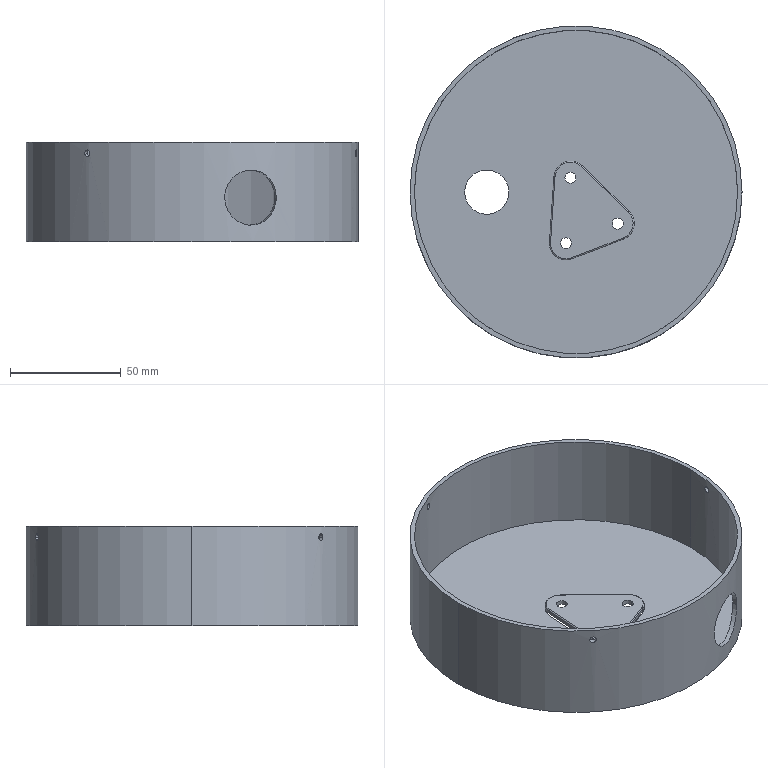Part | SolidWorks | features ICE 7, CirPattern 1, Cut 1, Extrusion 1, Fillet 1 | 2 solids | 46 faces | box 150 x 150 x 45 mm | volume 73548 mm3 | cylinder 31 | plane 11 | torus 4 | commonest cylinder face diameters 15 x8 3 x6 5 x6 1 x3 20 x2 25 x2